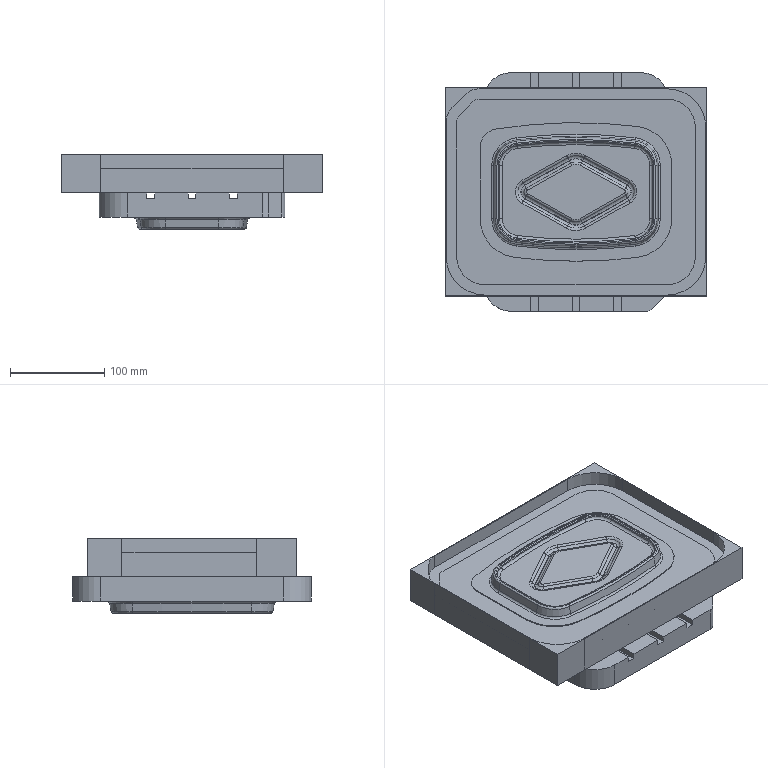Part | 4 solids | 501 faces | box 278.144 x 254.144 x 79 mm | volume 3132025 mm3 | plane 210 | cylinder 187 | torus 76 | cone 22 | spline 6 | commonest cylinder face diameters 2 x47 8 x25 6.171 x16 7.78 x16 56.68 x12 60 x9